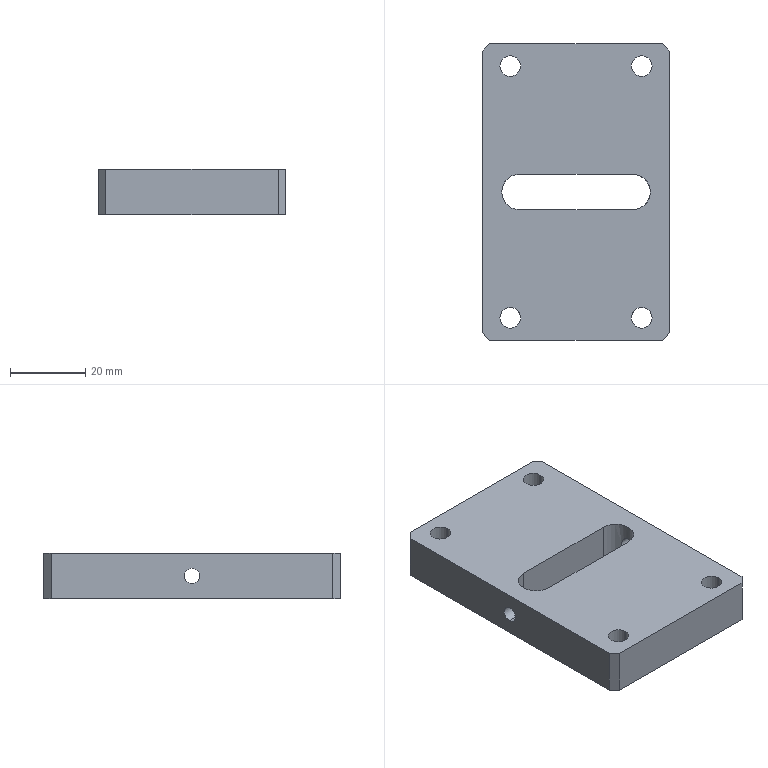Part | SolidWorks | features HoleWzd 3, Chamfer 1, Extrusion 1 | 1 solid | 39 faces | box 50 x 79 x 12 mm | volume 40495 mm3 | cylinder 23 | plane 16 | commonest cylinder face diameters 5.5 x8 10 x8 4.2 x4 9.5 x3
STEP:
#1=CARTESIAN_POINT('',(25.,0.,-2.1));
#2=VERTEX_POINT('',#1);
#3=CARTESIAN_POINT('',(25.,0.,2.1));
#4=VERTEX_POINT('',#3);
#5=CARTESIAN_POINT('',(25.,0.,0.));
#6=DIRECTION('',(-1.,0.,0.));
#7=DIRECTION('',(0.,0.,1.));
#8=AXIS2_PLACEMENT_3D('',#5,#6,#7);
#9=CIRCLE('',#8,2.1);
#10=EDGE_CURVE('',#2,#4,#9,.T.);
#11=ORIENTED_EDGE('',*,*,#10,.F.);
#12=CARTESIAN_POINT('',(19.75,0.,-2.1));
#13=VERTEX_POINT('',#12);
#14=CARTESIAN_POINT('',(-25.,0.,-2.1));
#15=DIRECTION('',(-1.,0.,0.));
#16=VECTOR('',#15,1000.);
#17=LINE('',#14,#16);
#18=EDGE_CURVE('',#2,#13,#17,.T.);
#19=ORIENTED_EDGE('',*,*,#18,.T.);
#20=CARTESIAN_POINT('',(19.75,0.,2.1));
#21=VERTEX_POINT('',#20);
#22=CARTESIAN_POINT('',(19.75,0.,2.1));
#23=CARTESIAN_POINT('',(19.75,-0.1407,2.1));
#24=CARTESIAN_POINT('',(19.744,-0.2787,2.086));
#25=CARTESIAN_POINT('',(19.72,-0.5497,2.031));
#26=CARTESIAN_POINT('',(19.702,-0.6841,1.99));
#27=CARTESIAN_POINT('',(19.658,-0.9378,1.884));
#28=CARTESIAN_POINT('',(19.632,-1.058,1.819));
#29=CARTESIAN_POINT('',(19.574,-1.285,1.667));
#30=CARTESIAN_POINT('',(19.543,-1.391,1.579));
#31=CARTESIAN_POINT('',(19.449,-1.677,1.292));
#32=CARTESIAN_POINT('',(19.384,-1.832,1.062));
#33=CARTESIAN_POINT('',(19.313,-1.99,0.684));
#34=CARTESIAN_POINT('',(19.294,-2.031,0.55));
#35=CARTESIAN_POINT('',(19.267,-2.086,0.2781));
#36=CARTESIAN_POINT('',(19.261,-2.1,0.1406));
#37=CARTESIAN_POINT('',(19.261,-2.1,-0.1376));
#38=CARTESIAN_POINT('',(19.268,-2.086,-0.2786));
#39=CARTESIAN_POINT('',(19.294,-2.031,-0.5497));
#40=CARTESIAN_POINT('',(19.313,-1.991,-0.6823));
#41=CARTESIAN_POINT('',(19.361,-1.884,-0.9374));
#42=CARTESIAN_POINT('',(19.388,-1.819,-1.057));
#43=CARTESIAN_POINT('',(19.448,-1.668,-1.283));
#44=CARTESIAN_POINT('',(19.481,-1.58,-1.39));
#45=CARTESIAN_POINT('',(19.544,-1.389,-1.581));
#46=CARTESIAN_POINT('',(19.575,-1.284,-1.667));
#47=CARTESIAN_POINT('',(19.632,-1.057,-1.82));
#48=CARTESIAN_POINT('',(19.659,-0.9355,-1.885));
#49=CARTESIAN_POINT('',(19.724,-0.5571,-2.043));
#50=CARTESIAN_POINT('',(19.75,-0.2773,-2.1));
#51=CARTESIAN_POINT('',(19.75,0.,-2.1));
#52=B_SPLINE_CURVE_WITH_KNOTS('',3,(#22,#23,#24,#25,#26,#27,#28,#29,#30,#31,#32,#33,#34,#35,#36,#37,#38,#39,#40,#41,#42,#43,#44,#45,#46,#47,#48,#49,#50,#51),.UNSPECIFIED.,.F.,.F.,(4,2,2,2,2,2,2,2,2,2,2,2,2,2,4),(0.,0.0004158,0.0008316,0.001247,0.001663,0.002495,0.002911,0.003326,0.003742,0.004158,0.004574,0.00499,0.005405,0.005821,0.006653),.UNSPECIFIED.);
#53=EDGE_CURVE('',#21,#13,#52,.T.);
#54=ORIENTED_EDGE('',*,*,#53,.F.);
#55=CARTESIAN_POINT('',(-25.,0.,2.1));
#56=DIRECTION('',(-1.,0.,0.));
#57=VECTOR('',#56,1000.);
#58=LINE('',#55,#57);
#59=EDGE_CURVE('',#4,#21,#58,.T.);
#60=ORIENTED_EDGE('',*,*,#59,.F.);
#61=EDGE_LOOP('',(#11,#19,#54,#60));
#62=FACE_OUTER_BOUND('',#61,.T.);
#63=CARTESIAN_POINT('',(-25.,0.,0.));
#64=DIRECTION('',(-1.,0.,0.));
#65=DIRECTION('',(0.,0.,1.));
#66=AXIS2_PLACEMENT_3D('',#63,#64,#65);
#67=CYLINDRICAL_SURFACE('',#66,2.1);
#68=ADVANCED_FACE('',(#62),#67,.F.);
#69=CARTESIAN_POINT('',(-19.75,0.,-2.1));
#70=VERTEX_POINT('',#69);
#71=CARTESIAN_POINT('',(-19.75,0.,2.1));
#72=VERTEX_POINT('',#71);
#73=CARTESIAN_POINT('',(-19.75,0.,-2.1));
#74=CARTESIAN_POINT('',(-19.75,-0.1385,-2.1));
#75=CARTESIAN_POINT('',(-19.744,-0.2793,-2.086));
#76=CARTESIAN_POINT('',(-19.72,-0.5513,-2.031));
#77=CARTESIAN_POINT('',(-19.702,-0.6829,-1.991));
#78=CARTESIAN_POINT('',(-19.636,-1.065,-1.831));
#79=CARTESIAN_POINT('',(-19.575,-1.294,-1.676));
#80=CARTESIAN_POINT('',(-19.48,-1.583,-1.387));
#81=CARTESIAN_POINT('',(-19.448,-1.668,-1.283));
#82=CARTESIAN_POINT('',(-19.389,-1.819,-1.057));
#83=CARTESIAN_POINT('',(-19.36,-1.885,-0.9352));
#84=CARTESIAN_POINT('',(-19.313,-1.991,-0.6828));
#85=CARTESIAN_POINT('',(-19.294,-2.031,-0.552));
#86=CARTESIAN_POINT('',(-19.268,-2.086,-0.2803));
#87=CARTESIAN_POINT('',(-19.261,-2.1,-0.1395));
#88=CARTESIAN_POINT('',(-19.261,-2.1,0.276));
#89=CARTESIAN_POINT('',(-19.289,-2.044,0.5553));
#90=CARTESIAN_POINT('',(-19.36,-1.885,0.935));
#91=CARTESIAN_POINT('',(-19.388,-1.82,1.057));
#92=CARTESIAN_POINT('',(-19.448,-1.668,1.283));
#93=CARTESIAN_POINT('',(-19.48,-1.582,1.387));
#94=CARTESIAN_POINT('',(-19.575,-1.293,1.677));
#95=CARTESIAN_POINT('',(-19.636,-1.066,1.831));
#96=CARTESIAN_POINT('',(-19.702,-0.6831,1.991));
#97=CARTESIAN_POINT('',(-19.72,-0.5517,2.031));
#98=CARTESIAN_POINT('',(-19.744,-0.2812,2.086));
#99=CARTESIAN_POINT('',(-19.75,-0.1406,2.1));
#100=CARTESIAN_POINT('',(-19.75,0.,2.1));
#101=B_SPLINE_CURVE_WITH_KNOTS('',3,(#73,#74,#75,#76,#77,#78,#79,#80,#81,#82,#83,#84,#85,#86,#87,#88,#89,#90,#91,#92,#93,#94,#95,#96,#97,#98,#99,#100),.UNSPECIFIED.,.F.,.F.,(4,2,2,2,2,2,2,2,2,2,2,2,2,4),(0.006653,0.007068,0.007483,0.008314,0.00873,0.009145,0.00956,0.009976,0.01081,0.01122,0.01164,0.01247,0.01288,0.0133),.UNSPECIFIED.);
#102=EDGE_CURVE('',#70,#72,#101,.T.);
#103=ORIENTED_EDGE('',*,*,#102,.F.);
#104=CARTESIAN_POINT('',(-25.,0.,-2.1));
#105=VERTEX_POINT('',#104);
#106=CARTESIAN_POINT('',(-25.,0.,-2.1));
#107=DIRECTION('',(-1.,0.,0.));
#108=VECTOR('',#107,1000.);
#109=LINE('',#106,#108);
#110=EDGE_CURVE('',#70,#105,#109,.T.);
#111=ORIENTED_EDGE('',*,*,#110,.T.);
#112=CARTESIAN_POINT('',(-25.,0.,2.1));
#113=VERTEX_POINT('',#112);
#114=CARTESIAN_POINT('',(-25.,0.,0.));
#115=DIRECTION('',(-1.,0.,0.));
#116=DIRECTION('',(0.,0.,1.));
#117=AXIS2_PLACEMENT_3D('',#114,#115,#116);
#118=CIRCLE('',#117,2.1);
#119=EDGE_CURVE('',#105,#113,#118,.T.);
#120=ORIENTED_EDGE('',*,*,#119,.T.);
#121=CARTESIAN_POINT('',(-25.,0.,2.1));
#122=DIRECTION('',(-1.,0.,0.));
#123=VECTOR('',#122,1000.);
#124=LINE('',#121,#123);
#125=EDGE_CURVE('',#72,#113,#124,.T.);
#126=ORIENTED_EDGE('',*,*,#125,.F.);
#127=EDGE_LOOP('',(#103,#111,#120,#126));
#128=FACE_OUTER_BOUND('',#127,.T.);
#129=CARTESIAN_POINT('',(-25.,0.,0.));
#130=DIRECTION('',(-1.,0.,0.));
#131=DIRECTION('',(0.,0.,1.));
#132=AXIS2_PLACEMENT_3D('',#129,#130,#131);
#133=CYLINDRICAL_SURFACE('',#132,2.1);
#134=ADVANCED_FACE('',(#128),#133,.F.);
#135=CARTESIAN_POINT('',(-12.5,33.5,-0.3));
#136=VERTEX_POINT('',#135);
#137=CARTESIAN_POINT('',(-22.5,33.5,-0.3));
#138=VERTEX_POINT('',#137);
#139=CARTESIAN_POINT('',(-17.5,33.5,-0.3));
#140=DIRECTION('',(0.,0.,-1.));
#141=DIRECTION('',(-1.,0.,0.));
#142=AXIS2_PLACEMENT_3D('',#139,#140,#141);
#143=CIRCLE('',#142,5.);
#144=EDGE_CURVE('',#136,#138,#143,.T.);
#145=ORIENTED_EDGE('',*,*,#144,.F.);
#146=CARTESIAN_POINT('',(-12.5,33.5,-6.));
#147=VERTEX_POINT('',#146);
#148=CARTESIAN_POINT('',(-12.5,33.5,-6.));
#149=DIRECTION('',(0.,0.,-1.));
#150=VECTOR('',#149,1000.);
#151=LINE('',#148,#150);
#152=EDGE_CURVE('',#136,#147,#151,.T.);
#153=ORIENTED_EDGE('',*,*,#152,.T.);
#154=CARTESIAN_POINT('',(-22.5,33.5,-6.));
#155=VERTEX_POINT('',#154);
#156=CARTESIAN_POINT('',(-17.5,33.5,-6.));
#157=DIRECTION('',(0.,0.,-1.));
#158=DIRECTION('',(-1.,0.,0.));
#159=AXIS2_PLACEMENT_3D('',#156,#157,#158);
#160=CIRCLE('',#159,5.);
#161=EDGE_CURVE('',#147,#155,#160,.T.);
#162=ORIENTED_EDGE('',*,*,#161,.T.);
#163=CARTESIAN_POINT('',(-22.5,33.5,-6.));
#164=DIRECTION('',(0.,0.,-1.));
#165=VECTOR('',#164,1000.);
#166=LINE('',#163,#165);
#167=EDGE_CURVE('',#138,#155,#166,.T.);
#168=ORIENTED_EDGE('',*,*,#167,.F.);
#169=EDGE_LOOP('',(#145,#153,#162,#168));
#170=FACE_OUTER_BOUND('',#169,.T.);
#171=CARTESIAN_POINT('',(-17.5,33.5,-6.));
#172=DIRECTION('',(0.,0.,-1.));
#173=DIRECTION('',(-1.,0.,0.));
#174=AXIS2_PLACEMENT_3D('',#171,#172,#173);
#175=CYLINDRICAL_SURFACE('',#174,5.);
#176=ADVANCED_FACE('',(#170),#175,.F.);
#177=CARTESIAN_POINT('',(-14.75,33.5,6.));
#178=VERTEX_POINT('',#177);
#179=CARTESIAN_POINT('',(-20.25,33.5,6.));
#180=VERTEX_POINT('',#179);
#181=CARTESIAN_POINT('',(-17.5,33.5,6.));
#182=DIRECTION('',(0.,0.,-1.));
#183=DIRECTION('',(-1.,0.,0.));
#184=AXIS2_PLACEMENT_3D('',#181,#182,#183);
#185=CIRCLE('',#184,2.75);
#186=EDGE_CURVE('',#178,#180,#185,.T.);
#187=ORIENTED_EDGE('',*,*,#186,.F.);
#188=CARTESIAN_POINT('',(-14.75,33.5,-0.3));
#189=VERTEX_POINT('',#188);
#190=CARTESIAN_POINT('',(-14.75,33.5,-6.));
#191=DIRECTION('',(0.,0.,-1.));
#192=VECTOR('',#191,1000.);
#193=LINE('',#190,#192);
#194=EDGE_CURVE('',#178,#189,#193,.T.);
#195=ORIENTED_EDGE('',*,*,#194,.T.);
#196=CARTESIAN_POINT('',(-20.25,33.5,-0.3));
#197=VERTEX_POINT('',#196);
#198=CARTESIAN_POINT('',(-17.5,33.5,-0.3));
#199=DIRECTION('',(0.,0.,-1.));
#200=DIRECTION('',(-1.,0.,0.));
#201=AXIS2_PLACEMENT_3D('',#198,#199,#200);
#202=CIRCLE('',#201,2.75);
#203=EDGE_CURVE('',#189,#197,#202,.T.);
#204=ORIENTED_EDGE('',*,*,#203,.T.);
#205=CARTESIAN_POINT('',(-20.25,33.5,-6.));
#206=DIRECTION('',(0.,0.,-1.));
#207=VECTOR('',#206,1000.);
#208=LINE('',#205,#207);
#209=EDGE_CURVE('',#180,#197,#208,.T.);
#210=ORIENTED_EDGE('',*,*,#209,.F.);
#211=EDGE_LOOP('',(#187,#195,#204,#210));
#212=FACE_OUTER_BOUND('',#211,.T.);
#213=CARTESIAN_POINT('',(-17.5,33.5,-6.));
#214=DIRECTION('',(0.,0.,-1.));
#215=DIRECTION('',(-1.,0.,0.));
#216=AXIS2_PLACEMENT_3D('',#213,#214,#215);
#217=CYLINDRICAL_SURFACE('',#216,2.75);
#218=ADVANCED_FACE('',(#212),#217,.F.);
#219=CARTESIAN_POINT('',(22.5,33.5,-0.3));
#220=VERTEX_POINT('',#219);
#221=CARTESIAN_POINT('',(12.5,33.5,-0.3));
#222=VERTEX_POINT('',#221);
#223=CARTESIAN_POINT('',(17.5,33.5,-0.3));
#224=DIRECTION('',(0.,0.,-1.));
#225=DIRECTION('',(-1.,0.,0.));
#226=AXIS2_PLACEMENT_3D('',#223,#224,#225);
#227=CIRCLE('',#226,5.);
#228=EDGE_CURVE('',#220,#222,#227,.T.);
#229=ORIENTED_EDGE('',*,*,#228,.F.);
#230=CARTESIAN_POINT('',(22.5,33.5,-6.));
#231=VERTEX_POINT('',#230);
#232=CARTESIAN_POINT('',(22.5,33.5,-6.));
#233=DIRECTION('',(0.,0.,-1.));
#234=VECTOR('',#233,1000.);
#235=LINE('',#232,#234);
#236=EDGE_CURVE('',#220,#231,#235,.T.);
#237=ORIENTED_EDGE('',*,*,#236,.T.);
#238=CARTESIAN_POINT('',(12.5,33.5,-6.));
#239=VERTEX_POINT('',#238);
#240=CARTESIAN_POINT('',(17.5,33.5,-6.));
#241=DIRECTION('',(0.,0.,-1.));
#242=DIRECTION('',(-1.,0.,0.));
#243=AXIS2_PLACEMENT_3D('',#240,#241,#242);
#244=CIRCLE('',#243,5.);
#245=EDGE_CURVE('',#231,#239,#244,.T.);
#246=ORIENTED_EDGE('',*,*,#245,.T.);
#247=CARTESIAN_POINT('',(12.5,33.5,-6.));
#248=DIRECTION('',(0.,0.,-1.));
#249=VECTOR('',#248,1000.);
#250=LINE('',#247,#249);
#251=EDGE_CURVE('',#222,#239,#250,.T.);
#252=ORIENTED_EDGE('',*,*,#251,.F.);
#253=EDGE_LOOP('',(#229,#237,#246,#252));
#254=FACE_OUTER_BOUND('',#253,.T.);
#255=CARTESIAN_POINT('',(17.5,33.5,-6.));
#256=DIRECTION('',(0.,0.,-1.));
#257=DIRECTION('',(-1.,0.,0.));
#258=AXIS2_PLACEMENT_3D('',#255,#256,#257);
#259=CYLINDRICAL_SURFACE('',#258,5.);
#260=ADVANCED_FACE('',(#254),#259,.F.);
#261=CARTESIAN_POINT('',(20.25,33.5,6.));
#262=VERTEX_POINT('',#261);
#263=CARTESIAN_POINT('',(14.75,33.5,6.));
#264=VERTEX_POINT('',#263);
#265=CARTESIAN_POINT('',(17.5,33.5,6.));
#266=DIRECTION('',(0.,0.,-1.));
#267=DIRECTION('',(-1.,0.,0.));
#268=AXIS2_PLACEMENT_3D('',#265,#266,#267);
#269=CIRCLE('',#268,2.75);
#270=EDGE_CURVE('',#262,#264,#269,.T.);
#271=ORIENTED_EDGE('',*,*,#270,.F.);
#272=CARTESIAN_POINT('',(20.25,33.5,-0.3));
#273=VERTEX_POINT('',#272);
#274=CARTESIAN_POINT('',(20.25,33.5,-6.));
#275=DIRECTION('',(0.,0.,-1.));
#276=VECTOR('',#275,1000.);
#277=LINE('',#274,#276);
#278=EDGE_CURVE('',#262,#273,#277,.T.);
#279=ORIENTED_EDGE('',*,*,#278,.T.);
#280=CARTESIAN_POINT('',(14.75,33.5,-0.3));
#281=VERTEX_POINT('',#280);
#282=CARTESIAN_POINT('',(17.5,33.5,-0.3));
#283=DIRECTION('',(0.,0.,-1.));
#284=DIRECTION('',(-1.,0.,0.));
#285=AXIS2_PLACEMENT_3D('',#282,#283,#284);
#286=CIRCLE('',#285,2.75);
#287=EDGE_CURVE('',#273,#281,#286,.T.);
#288=ORIENTED_EDGE('',*,*,#287,.T.);
#289=CARTESIAN_POINT('',(14.75,33.5,-6.));
#290=DIRECTION('',(0.,0.,-1.));
#291=VECTOR('',#290,1000.);
#292=LINE('',#289,#291);
#293=EDGE_CURVE('',#264,#281,#292,.T.);
#294=ORIENTED_EDGE('',*,*,#293,.F.);
#295=EDGE_LOOP('',(#271,#279,#288,#294));
#296=FACE_OUTER_BOUND('',#295,.T.);
#297=CARTESIAN_POINT('',(17.5,33.5,-6.));
#298=DIRECTION('',(0.,0.,-1.));
#299=DIRECTION('',(-1.,0.,0.));
#300=AXIS2_PLACEMENT_3D('',#297,#298,#299);
#301=CYLINDRICAL_SURFACE('',#300,2.75);
#302=ADVANCED_FACE('',(#296),#301,.F.);
#303=CARTESIAN_POINT('',(-12.5,-33.5,-0.3));
#304=VERTEX_POINT('',#303);
#305=CARTESIAN_POINT('',(-22.5,-33.5,-0.3));
#306=VERTEX_POINT('',#305);
#307=CARTESIAN_POINT('',(-17.5,-33.5,-0.3));
#308=DIRECTION('',(0.,0.,-1.));
#309=DIRECTION('',(-1.,0.,0.));
#310=AXIS2_PLACEMENT_3D('',#307,#308,#309);
#311=CIRCLE('',#310,5.);
#312=EDGE_CURVE('',#304,#306,#311,.T.);
#313=ORIENTED_EDGE('',*,*,#312,.F.);
#314=CARTESIAN_POINT('',(-12.5,-33.5,-6.));
#315=VERTEX_POINT('',#314);
#316=CARTESIAN_POINT('',(-12.5,-33.5,-6.));
#317=DIRECTION('',(0.,0.,-1.));
#318=VECTOR('',#317,1000.);
#319=LINE('',#316,#318);
#320=EDGE_CURVE('',#304,#315,#319,.T.);
#321=ORIENTED_EDGE('',*,*,#320,.T.);
#322=CARTESIAN_POINT('',(-22.5,-33.5,-6.));
#323=VERTEX_POINT('',#322);
#324=CARTESIAN_POINT('',(-17.5,-33.5,-6.));
#325=DIRECTION('',(0.,0.,-1.));
#326=DIRECTION('',(-1.,0.,0.));
#327=AXIS2_PLACEMENT_3D('',#324,#325,#326);
#328=CIRCLE('',#327,5.);
#329=EDGE_CURVE('',#315,#323,#328,.T.);
#330=ORIENTED_EDGE('',*,*,#329,.T.);
#331=CARTESIAN_POINT('',(-22.5,-33.5,-6.));
#332=DIRECTION('',(0.,0.,-1.));
#333=VECTOR('',#332,1000.);
#334=LINE('',#331,#333);
#335=EDGE_CURVE('',#306,#323,#334,.T.);
#336=ORIENTED_EDGE('',*,*,#335,.F.);
#337=EDGE_LOOP('',(#313,#321,#330,#336));
#338=FACE_OUTER_BOUND('',#337,.T.);
#339=CARTESIAN_POINT('',(-17.5,-33.5,-6.));
#340=DIRECTION('',(0.,0.,-1.));
#341=DIRECTION('',(-1.,0.,0.));
#342=AXIS2_PLACEMENT_3D('',#339,#340,#341);
#343=CYLINDRICAL_SURFACE('',#342,5.);
#344=ADVANCED_FACE('',(#338),#343,.F.);
#345=CARTESIAN_POINT('',(-14.75,-33.5,6.));
#346=VERTEX_POINT('',#345);
#347=CARTESIAN_POINT('',(-20.25,-33.5,6.));
#348=VERTEX_POINT('',#347);
#349=CARTESIAN_POINT('',(-17.5,-33.5,6.));
#350=DIRECTION('',(0.,0.,-1.));
#351=DIRECTION('',(-1.,0.,0.));
#352=AXIS2_PLACEMENT_3D('',#349,#350,#351);
#353=CIRCLE('',#352,2.75);
#354=EDGE_CURVE('',#346,#348,#353,.T.);
#355=ORIENTED_EDGE('',*,*,#354,.F.);
#356=CARTESIAN_POINT('',(-14.75,-33.5,-0.3));
#357=VERTEX_POINT('',#356);
#358=CARTESIAN_POINT('',(-14.75,-33.5,-6.));
#359=DIRECTION('',(0.,0.,-1.));
#360=VECTOR('',#359,1000.);
#361=LINE('',#358,#360);
#362=EDGE_CURVE('',#346,#357,#361,.T.);
#363=ORIENTED_EDGE('',*,*,#362,.T.);
#364=CARTESIAN_POINT('',(-20.25,-33.5,-0.3));
#365=VERTEX_POINT('',#364);
#366=CARTESIAN_POINT('',(-17.5,-33.5,-0.3));
#367=DIRECTION('',(0.,0.,-1.));
#368=DIRECTION('',(-1.,0.,0.));
#369=AXIS2_PLACEMENT_3D('',#366,#367,#368);
#370=CIRCLE('',#369,2.75);
#371=EDGE_CURVE('',#357,#365,#370,.T.);
#372=ORIENTED_EDGE('',*,*,#371,.T.);
#373=CARTESIAN_POINT('',(-20.25,-33.5,-6.));
#374=DIRECTION('',(0.,0.,-1.));
#375=VECTOR('',#374,1000.);
#376=LINE('',#373,#375);
#377=EDGE_CURVE('',#348,#365,#376,.T.);
#378=ORIENTED_EDGE('',*,*,#377,.F.);
#379=EDGE_LOOP('',(#355,#363,#372,#378));
#380=FACE_OUTER_BOUND('',#379,.T.);
#381=CARTESIAN_POINT('',(-17.5,-33.5,-6.));
#382=DIRECTION('',(0.,0.,-1.));
#383=DIRECTION('',(-1.,0.,0.));
#384=AXIS2_PLACEMENT_3D('',#381,#382,#383);
#385=CYLINDRICAL_SURFACE('',#384,2.75);
#386=ADVANCED_FACE('',(#380),#385,.F.);
#387=CARTESIAN_POINT('',(22.5,-33.5,-0.3));
#388=VERTEX_POINT('',#387);
#389=CARTESIAN_POINT('',(12.5,-33.5,-0.3));
#390=VERTEX_POINT('',#389);
#391=CARTESIAN_POINT('',(17.5,-33.5,-0.3));
#392=DIRECTION('',(0.,0.,-1.));
#393=DIRECTION('',(-1.,0.,0.));
#394=AXIS2_PLACEMENT_3D('',#391,#392,#393);
#395=CIRCLE('',#394,5.);
#396=EDGE_CURVE('',#388,#390,#395,.T.);
#397=ORIENTED_EDGE('',*,*,#396,.F.);
#398=CARTESIAN_POINT('',(22.5,-33.5,-6.));
#399=VERTEX_POINT('',#398);
#400=CARTESIAN_POINT('',(22.5,-33.5,-6.));
#401=DIRECTION('',(0.,0.,-1.));
#402=VECTOR('',#401,1000.);
#403=LINE('',#400,#402);
#404=EDGE_CURVE('',#388,#399,#403,.T.);
#405=ORIENTED_EDGE('',*,*,#404,.T.);
#406=CARTESIAN_POINT('',(12.5,-33.5,-6.));
#407=VERTEX_POINT('',#406);
#408=CARTESIAN_POINT('',(17.5,-33.5,-6.));
#409=DIRECTION('',(0.,0.,-1.));
#410=DIRECTION('',(-1.,0.,0.));
#411=AXIS2_PLACEMENT_3D('',#408,#409,#410);
#412=CIRCLE('',#411,5.);
#413=EDGE_CURVE('',#399,#407,#412,.T.);
#414=ORIENTED_EDGE('',*,*,#413,.T.);
#415=CARTESIAN_POINT('',(12.5,-33.5,-6.));
#416=DIRECTION('',(0.,0.,-1.));
#417=VECTOR('',#416,1000.);
#418=LINE('',#415,#417);
#419=EDGE_CURVE('',#390,#407,#418,.T.);
#420=ORIENTED_EDGE('',*,*,#419,.F.);
#421=EDGE_LOOP('',(#397,#405,#414,#420));
#422=FACE_OUTER_BOUND('',#421,.T.);
#423=CARTESIAN_POINT('',(17.5,-33.5,-6.));
#424=DIRECTION('',(0.,0.,-1.));
#425=DIRECTION('',(-1.,0.,0.));
#426=AXIS2_PLACEMENT_3D('',#423,#424,#425);
#427=CYLINDRICAL_SURFACE('',#426,5.);
#428=ADVANCED_FACE('',(#422),#427,.F.);
#429=CARTESIAN_POINT('',(20.25,-33.5,6.));
#430=VERTEX_POINT('',#429);
#431=CARTESIAN_POINT('',(14.75,-33.5,6.));
#432=VERTEX_POINT('',#431);
#433=CARTESIAN_POINT('',(17.5,-33.5,6.));
#434=DIRECTION('',(0.,0.,-1.));
#435=DIRECTION('',(-1.,0.,0.));
#436=AXIS2_PLACEMENT_3D('',#433,#434,#435);
#437=CIRCLE('',#436,2.75);
#438=EDGE_CURVE('',#430,#432,#437,.T.);
#439=ORIENTED_EDGE('',*,*,#438,.F.);
#440=CARTESIAN_POINT('',(20.25,-33.5,-0.3));
#441=VERTEX_POINT('',#440);
#442=CARTESIAN_POINT('',(20.25,-33.5,-6.));
#443=DIRECTION('',(0.,0.,-1.));
#444=VECTOR('',#443,1000.);
#445=LINE('',#442,#444);
#446=EDGE_CURVE('',#430,#441,#445,.T.);
#447=ORIENTED_EDGE('',*,*,#446,.T.);
#448=CARTESIAN_POINT('',(14.75,-33.5,-0.3));
#449=VERTEX_POINT('',#448);
#450=CARTESIAN_POINT('',(17.5,-33.5,-0.3));
#451=DIRECTION('',(0.,0.,-1.));
#452=DIRECTION('',(-1.,0.,0.));
#453=AXIS2_PLACEMENT_3D('',#450,#451,#452);
#454=CIRCLE('',#453,2.75);
#455=EDGE_CURVE('',#441,#449,#454,.T.);
#456=ORIENTED_EDGE('',*,*,#455,.T.);
#457=CARTESIAN_POINT('',(14.75,-33.5,-6.));
#458=DIRECTION('',(0.,0.,-1.));
#459=VECTOR('',#458,1000.);
#460=LINE('',#457,#459);
#461=EDGE_CURVE('',#432,#449,#460,.T.);
#462=ORIENTED_EDGE('',*,*,#461,.F.);
#463=EDGE_LOOP('',(#439,#447,#456,#462));
#464=FACE_OUTER_BOUND('',#463,.T.);
#465=CARTESIAN_POINT('',(17.5,-33.5,-6.));
#466=DIRECTION('',(0.,0.,-1.));
#467=DIRECTION('',(-1.,0.,0.));
#468=AXIS2_PLACEMENT_3D('',#465,#466,#467);
#469=CYLINDRICAL_SURFACE('',#468,2.75);
#470=ADVANCED_FACE('',(#464),#469,.F.);
#471=CARTESIAN_POINT('',(-19.75,0.,6.));
#472=VERTEX_POINT('',#471);
#473=CARTESIAN_POINT('',(-15.,4.75,6.));
#474=VERTEX_POINT('',#473);
#475=CARTESIAN_POINT('',(-15.,0.,6.));
#476=DIRECTION('',(0.,0.,-1.));
#477=DIRECTION('',(-1.,0.,0.));
#478=AXIS2_PLACEMENT_3D('',#475,#476,#477);
#479=CIRCLE('',#478,4.75);
#480=EDGE_CURVE('',#472,#474,#479,.T.);
#481=ORIENTED_EDGE('',*,*,#480,.F.);
#482=CARTESIAN_POINT('',(-19.75,0.,-6.));
#483=DIRECTION('',(0.,0.,-1.));
#484=VECTOR('',#483,1000.);
#485=LINE('',#482,#484);
#486=EDGE_CURVE('',#472,#72,#485,.T.);
#487=ORIENTED_EDGE('',*,*,#486,.T.);
#488=CARTESIAN_POINT('',(-19.75,0.,2.1));
#489=CARTESIAN_POINT('',(-19.75,0.1407,2.1));
#490=CARTESIAN_POINT('',(-19.744,0.2787,2.086));
#491=CARTESIAN_POINT('',(-19.72,0.5497,2.031));
#492=CARTESIAN_POINT('',(-19.702,0.6841,1.99));
#493=CARTESIAN_POINT('',(-19.658,0.9378,1.884));
#494=CARTESIAN_POINT('',(-19.632,1.058,1.819));
#495=CARTESIAN_POINT('',(-19.574,1.285,1.667));
#496=CARTESIAN_POINT('',(-19.543,1.391,1.579));
#497=CARTESIAN_POINT('',(-19.449,1.677,1.292));
#498=CARTESIAN_POINT('',(-19.384,1.832,1.062));
#499=CARTESIAN_POINT('',(-19.313,1.99,0.684));
#500=CARTESIAN_POINT('',(-19.294,2.031,0.55));
#501=CARTESIAN_POINT('',(-19.267,2.086,0.2781));
#502=CARTESIAN_POINT('',(-19.261,2.1,0.1406));
#503=CARTESIAN_POINT('',(-19.261,2.1,-0.1376));
#504=CARTESIAN_POINT('',(-19.268,2.086,-0.2786));
#505=CARTESIAN_POINT('',(-19.294,2.031,-0.5497));
#506=CARTESIAN_POINT('',(-19.313,1.991,-0.6823));
#507=CARTESIAN_POINT('',(-19.361,1.884,-0.9374));
#508=CARTESIAN_POINT('',(-19.388,1.819,-1.057));
#509=CARTESIAN_POINT('',(-19.448,1.668,-1.283));
#510=CARTESIAN_POINT('',(-19.481,1.58,-1.39));
#511=CARTESIAN_POINT('',(-19.544,1.389,-1.581));
#512=CARTESIAN_POINT('',(-19.575,1.284,-1.667));
#513=CARTESIAN_POINT('',(-19.632,1.057,-1.82));
#514=CARTESIAN_POINT('',(-19.659,0.9355,-1.885));
#515=CARTESIAN_POINT('',(-19.724,0.5571,-2.043));
#516=CARTESIAN_POINT('',(-19.75,0.2773,-2.1));
#517=CARTESIAN_POINT('',(-19.75,0.,-2.1));
#518=B_SPLINE_CURVE_WITH_KNOTS('',3,(#488,#489,#490,#491,#492,#493,#494,#495,#496,#497,#498,#499,#500,#501,#502,#503,#504,#505,#506,#507,#508,#509,#510,#511,#512,#513,#514,#515,#516,#517),.UNSPECIFIED.,.F.,.F.,(4,2,2,2,2,2,2,2,2,2,2,2,2,2,4),(0.,0.0004158,0.0008316,0.001247,0.001663,0.002495,0.002911,0.003326,0.003742,0.004158,0.004574,0.00499,0.005405,0.005821,0.006653),.UNSPECIFIED.);
#519=EDGE_CURVE('',#72,#70,#518,.T.);
#520=ORIENTED_EDGE('',*,*,#519,.T.);
#521=CARTESIAN_POINT('',(-19.75,0.,-6.));
#522=VERTEX_POINT('',#521);
#523=CARTESIAN_POINT('',(-19.75,0.,-6.));
#524=DIRECTION('',(0.,0.,-1.));
#525=VECTOR('',#524,1000.);
#526=LINE('',#523,#525);
#527=EDGE_CURVE('',#70,#522,#526,.T.);
#528=ORIENTED_EDGE('',*,*,#527,.T.);
#529=CARTESIAN_POINT('',(-15.,4.75,-6.));
#530=VERTEX_POINT('',#529);
#531=CARTESIAN_POINT('',(-15.,0.,-6.));
#532=DIRECTION('',(0.,0.,-1.));
#533=DIRECTION('',(-1.,0.,0.));
#534=AXIS2_PLACEMENT_3D('',#531,#532,#533);
#535=CIRCLE('',#534,4.75);
#536=EDGE_CURVE('',#522,#530,#535,.T.);
#537=ORIENTED_EDGE('',*,*,#536,.T.);
#538=CARTESIAN_POINT('',(-15.,4.75,-6.));
#539=DIRECTION('',(0.,0.,-1.));
#540=VECTOR('',#539,1000.);
#541=LINE('',#538,#540);
#542=EDGE_CURVE('',#474,#530,#541,.T.);
#543=ORIENTED_EDGE('',*,*,#542,.F.);
#544=EDGE_LOOP('',(#481,#487,#520,#528,#537,#543));
#545=FACE_OUTER_BOUND('',#544,.T.);
#546=CARTESIAN_POINT('',(-15.,0.,-6.));
#547=DIRECTION('',(0.,0.,-1.));
#548=DIRECTION('',(-1.,0.,0.));
#549=AXIS2_PLACEMENT_3D('',#546,#547,#548);
#550=CYLINDRICAL_SURFACE('',#549,4.75);
#551=ADVANCED_FACE('',(#545),#550,.F.);
#552=CARTESIAN_POINT('',(25.,0.,0.));
#553=DIRECTION('',(-1.,0.,0.));
#554=DIRECTION('',(0.,0.,1.));
#555=AXIS2_PLACEMENT_3D('',#552,#553,#554);
#556=CIRCLE('',#555,2.1);
#557=EDGE_CURVE('',#4,#2,#556,.T.);
#558=ORIENTED_EDGE('',*,*,#557,.T.);
#559=ORIENTED_EDGE('',*,*,#10,.T.);
#560=EDGE_LOOP('',(#558,#559));
#561=FACE_BOUND('',#560,.T.);
#562=CARTESIAN_POINT('',(25.,-37.5,6.));
#563=VERTEX_POINT('',#562);
#564=CARTESIAN_POINT('',(25.,37.5,6.));
#565=VERTEX_POINT('',#564);
#566=CARTESIAN_POINT('',(25.,-39.5,6.));
#567=DIRECTION('',(0.,1.,0.));
#568=VECTOR('',#567,1000.);
#569=LINE('',#566,#568);
#570=EDGE_CURVE('',#563,#565,#569,.T.);
#571=ORIENTED_EDGE('',*,*,#570,.F.);
#572=CARTESIAN_POINT('',(25.,-37.5,-6.));
#573=VERTEX_POINT('',#572);
#574=CARTESIAN_POINT('',(25.,-37.5,6.));
#575=DIRECTION('',(0.,0.,-1.));
#576=VECTOR('',#575,1000.);
#577=LINE('',#574,#576);
#578=EDGE_CURVE('',#563,#573,#577,.T.);
#579=ORIENTED_EDGE('',*,*,#578,.T.);
#580=CARTESIAN_POINT('',(25.,37.5,-6.));
#581=VERTEX_POINT('',#580);
#582=CARTESIAN_POINT('',(25.,-39.5,-6.));
#583=DIRECTION('',(0.,1.,0.));
#584=VECTOR('',#583,1000.);
#585=LINE('',#582,#584);
#586=EDGE_CURVE('',#573,#581,#585,.T.);
#587=ORIENTED_EDGE('',*,*,#586,.T.);
#588=CARTESIAN_POINT('',(25.,37.5,6.));
#589=DIRECTION('',(0.,0.,1.));
#590=VECTOR('',#589,1000.);
#591=LINE('',#588,#590);
#592=EDGE_CURVE('',#581,#565,#591,.T.);
#593=ORIENTED_EDGE('',*,*,#592,.T.);
#594=EDGE_LOOP('',(#571,#579,#587,#593));
#595=FACE_OUTER_BOUND('',#594,.T.);
#596=CARTESIAN_POINT('',(25.,-39.5,6.));
#597=DIRECTION('',(-1.,0.,0.));
#598=DIRECTION('',(0.,0.,1.));
#599=AXIS2_PLACEMENT_3D('',#596,#597,#598);
#600=PLANE('',#599);
#601=ADVANCED_FACE('',(#561,#595),#600,.F.);
#602=CARTESIAN_POINT('',(23.,39.5,-6.));
#603=VERTEX_POINT('',#602);
#604=CARTESIAN_POINT('',(-23.,39.5,-6.));
#605=VERTEX_POINT('',#604);
#606=CARTESIAN_POINT('',(-25.,39.5,-6.));
#607=DIRECTION('',(-1.,0.,0.));
#608=VECTOR('',#607,1000.);
#609=LINE('',#606,#608);
#610=EDGE_CURVE('',#603,#605,#609,.T.);
#611=ORIENTED_EDGE('',*,*,#610,.T.);
#612=CARTESIAN_POINT('',(-23.,39.5,6.));
#613=VERTEX_POINT('',#612);
#614=CARTESIAN_POINT('',(-23.,39.5,6.));
#615=DIRECTION('',(0.,0.,1.));
#616=VECTOR('',#615,1000.);
#617=LINE('',#614,#616);
#618=EDGE_CURVE('',#605,#613,#617,.T.);
#619=ORIENTED_EDGE('',*,*,#618,.T.);
#620=CARTESIAN_POINT('',(23.,39.5,6.));
#621=VERTEX_POINT('',#620);
#622=CARTESIAN_POINT('',(-25.,39.5,6.));
#623=DIRECTION('',(-1.,0.,0.));
#624=VECTOR('',#623,1000.);
#625=LINE('',#622,#624);
#626=EDGE_CURVE('',#621,#613,#625,.T.);
#627=ORIENTED_EDGE('',*,*,#626,.F.);
#628=CARTESIAN_POINT('',(23.,39.5,6.));
#629=DIRECTION('',(0.,0.,-1.));
#630=VECTOR('',#629,1000.);
#631=LINE('',#628,#630);
#632=EDGE_CURVE('',#621,#603,#631,.T.);
#633=ORIENTED_EDGE('',*,*,#632,.T.);
#634=EDGE_LOOP('',(#611,#619,#627,#633));
#635=FACE_OUTER_BOUND('',#634,.T.);
#636=CARTESIAN_POINT('',(-25.,39.5,6.));
#637=DIRECTION('',(0.,-1.,0.));
#638=DIRECTION('',(0.,0.,-1.));
#639=AXIS2_PLACEMENT_3D('',#636,#637,#638);
#640=PLANE('',#639);
#641=ADVANCED_FACE('',(#635),#640,.F.);
#642=CARTESIAN_POINT('',(-25.,0.,0.));
#643=DIRECTION('',(-1.,0.,0.));
#644=DIRECTION('',(0.,0.,1.));
#645=AXIS2_PLACEMENT_3D('',#642,#643,#644);
#646=CIRCLE('',#645,2.1);
#647=EDGE_CURVE('',#113,#105,#646,.T.);
#648=ORIENTED_EDGE('',*,*,#647,.F.);
#649=ORIENTED_EDGE('',*,*,#119,.F.);
#650=EDGE_LOOP('',(#648,#649));
#651=FACE_BOUND('',#650,.T.);
#652=CARTESIAN_POINT('',(-25.,37.5,-6.));
#653=VERTEX_POINT('',#652);
#654=CARTESIAN_POINT('',(-25.,-37.5,-6.));
#655=VERTEX_POINT('',#654);
#656=CARTESIAN_POINT('',(-25.,-39.5,-6.));
#657=DIRECTION('',(0.,-1.,0.));
#658=VECTOR('',#657,1000.);
#659=LINE('',#656,#658);
#660=EDGE_CURVE('',#653,#655,#659,.T.);
#661=ORIENTED_EDGE('',*,*,#660,.T.);
#662=CARTESIAN_POINT('',(-25.,-37.5,6.));
#663=VERTEX_POINT('',#662);
#664=CARTESIAN_POINT('',(-25.,-37.5,6.));
#665=DIRECTION('',(0.,0.,1.));
#666=VECTOR('',#665,1000.);
#667=LINE('',#664,#666);
#668=EDGE_CURVE('',#655,#663,#667,.T.);
#669=ORIENTED_EDGE('',*,*,#668,.T.);
#670=CARTESIAN_POINT('',(-25.,37.5,6.));
#671=VERTEX_POINT('',#670);
#672=CARTESIAN_POINT('',(-25.,-39.5,6.));
#673=DIRECTION('',(0.,-1.,0.));
#674=VECTOR('',#673,1000.);
#675=LINE('',#672,#674);
#676=EDGE_CURVE('',#671,#663,#675,.T.);
#677=ORIENTED_EDGE('',*,*,#676,.F.);
#678=CARTESIAN_POINT('',(-25.,37.5,6.));
#679=DIRECTION('',(0.,0.,-1.));
#680=VECTOR('',#679,1000.);
#681=LINE('',#678,#680);
#682=EDGE_CURVE('',#671,#653,#681,.T.);
#683=ORIENTED_EDGE('',*,*,#682,.T.);
#684=EDGE_LOOP('',(#661,#669,#677,#683));
#685=FACE_OUTER_BOUND('',#684,.T.);
#686=CARTESIAN_POINT('',(-25.,-39.5,6.));
#687=DIRECTION('',(1.,0.,0.));
#688=DIRECTION('',(0.,0.,-1.));
#689=AXIS2_PLACEMENT_3D('',#686,#687,#688);
#690=PLANE('',#689);
#691=ADVANCED_FACE('',(#651,#685),#690,.F.);
#692=CARTESIAN_POINT('',(-23.,-39.5,-6.));
#693=VERTEX_POINT('',#692);
#694=CARTESIAN_POINT('',(23.,-39.5,-6.));
#695=VERTEX_POINT('',#694);
#696=CARTESIAN_POINT('',(-25.,-39.5,-6.));
#697=DIRECTION('',(1.,0.,0.));
#698=VECTOR('',#697,1000.);
#699=LINE('',#696,#698);
#700=EDGE_CURVE('',#693,#695,#699,.T.);
#701=ORIENTED_EDGE('',*,*,#700,.T.);
#702=CARTESIAN_POINT('',(23.,-39.5,6.));
#703=VERTEX_POINT('',#702);
#704=CARTESIAN_POINT('',(23.,-39.5,6.));
#705=DIRECTION('',(0.,0.,1.));
#706=VECTOR('',#705,1000.);
#707=LINE('',#704,#706);
#708=EDGE_CURVE('',#695,#703,#707,.T.);
#709=ORIENTED_EDGE('',*,*,#708,.T.);
#710=CARTESIAN_POINT('',(-23.,-39.5,6.));
#711=VERTEX_POINT('',#710);
#712=CARTESIAN_POINT('',(-25.,-39.5,6.));
#713=DIRECTION('',(1.,0.,0.));
#714=VECTOR('',#713,1000.);
#715=LINE('',#712,#714);
#716=EDGE_CURVE('',#711,#703,#715,.T.);
#717=ORIENTED_EDGE('',*,*,#716,.F.);
#718=CARTESIAN_POINT('',(-23.,-39.5,6.));
#719=DIRECTION('',(0.,0.,-1.));
#720=VECTOR('',#719,1000.);
#721=LINE('',#718,#720);
#722=EDGE_CURVE('',#711,#693,#721,.T.);
#723=ORIENTED_EDGE('',*,*,#722,.T.);
#724=EDGE_LOOP('',(#701,#709,#717,#723));
#725=FACE_OUTER_BOUND('',#724,.T.);
#726=CARTESIAN_POINT('',(-25.,-39.5,6.));
#727=DIRECTION('',(0.,1.,0.));
#728=DIRECTION('',(0.,0.,1.));
#729=AXIS2_PLACEMENT_3D('',#726,#727,#728);
#730=PLANE('',#729);
#731=ADVANCED_FACE('',(#725),#730,.F.);
#732=CARTESIAN_POINT('',(-17.5,33.5,6.));
#733=DIRECTION('',(0.,0.,-1.));
#734=DIRECTION('',(-1.,0.,0.));
#735=AXIS2_PLACEMENT_3D('',#732,#733,#734);
#736=CIRCLE('',#735,2.75);
#737=EDGE_CURVE('',#180,#178,#736,.T.);
#738=ORIENTED_EDGE('',*,*,#737,.T.);
#739=ORIENTED_EDGE('',*,*,#186,.T.);
#740=EDGE_LOOP('',(#738,#739));
#741=FACE_BOUND('',#740,.T.);
#742=CARTESIAN_POINT('',(17.5,33.5,6.));
#743=DIRECTION('',(0.,0.,-1.));
#744=DIRECTION('',(-1.,0.,0.));
#745=AXIS2_PLACEMENT_3D('',#742,#743,#744);
#746=CIRCLE('',#745,2.75);
#747=EDGE_CURVE('',#264,#262,#746,.T.);
#748=ORIENTED_EDGE('',*,*,#747,.T.);
#749=ORIENTED_EDGE('',*,*,#270,.T.);
#750=EDGE_LOOP('',(#748,#749));
#751=FACE_BOUND('',#750,.T.);
#752=CARTESIAN_POINT('',(-17.5,-33.5,6.));
#753=DIRECTION('',(0.,0.,-1.));
#754=DIRECTION('',(-1.,0.,0.));
#755=AXIS2_PLACEMENT_3D('',#752,#753,#754);
#756=CIRCLE('',#755,2.75);
#757=EDGE_CURVE('',#348,#346,#756,.T.);
#758=ORIENTED_EDGE('',*,*,#757,.T.);
#759=ORIENTED_EDGE('',*,*,#354,.T.);
#760=EDGE_LOOP('',(#758,#759));
#761=FACE_BOUND('',#760,.T.);
#762=CARTESIAN_POINT('',(17.5,-33.5,6.));
#763=DIRECTION('',(0.,0.,-1.));
#764=DIRECTION('',(-1.,0.,0.));
#765=AXIS2_PLACEMENT_3D('',#762,#763,#764);
#766=CIRCLE('',#765,2.75);
#767=EDGE_CURVE('',#432,#430,#766,.T.);
#768=ORIENTED_EDGE('',*,*,#767,.T.);
#769=ORIENTED_EDGE('',*,*,#438,.T.);
#770=EDGE_LOOP('',(#768,#769));
#771=FACE_BOUND('',#770,.T.);
#772=CARTESIAN_POINT('',(15.,4.75,6.));
#773=VERTEX_POINT('',#772);
#774=CARTESIAN_POINT('',(-15.,4.75,6.));
#775=DIRECTION('',(1.,0.,0.));
#776=VECTOR('',#775,1000.);
#777=LINE('',#774,#776);
#778=EDGE_CURVE('',#474,#773,#777,.T.);
#779=ORIENTED_EDGE('',*,*,#778,.T.);
#780=CARTESIAN_POINT('',(15.,-4.75,6.));
#781=VERTEX_POINT('',#780);
#782=CARTESIAN_POINT('',(15.,0.,6.));
#783=DIRECTION('',(0.,0.,-1.));
#784=DIRECTION('',(-1.,0.,0.));
#785=AXIS2_PLACEMENT_3D('',#782,#783,#784);
#786=CIRCLE('',#785,4.75);
#787=EDGE_CURVE('',#773,#781,#786,.T.);
#788=ORIENTED_EDGE('',*,*,#787,.T.);
#789=CARTESIAN_POINT('',(-15.,-4.75,6.));
#790=VERTEX_POINT('',#789);
#791=CARTESIAN_POINT('',(-15.,-4.75,6.));
#792=DIRECTION('',(1.,0.,0.));
#793=VECTOR('',#792,1000.);
#794=LINE('',#791,#793);
#795=EDGE_CURVE('',#790,#781,#794,.T.);
#796=ORIENTED_EDGE('',*,*,#795,.F.);
#797=CARTESIAN_POINT('',(-15.,0.,6.));
#798=DIRECTION('',(0.,0.,-1.));
#799=DIRECTION('',(-1.,0.,0.));
#800=AXIS2_PLACEMENT_3D('',#797,#798,#799);
#801=CIRCLE('',#800,4.75);
#802=EDGE_CURVE('',#790,#472,#801,.T.);
#803=ORIENTED_EDGE('',*,*,#802,.T.);
#804=ORIENTED_EDGE('',*,*,#480,.T.);
#805=EDGE_LOOP('',(#779,#788,#796,#803,#804));
#806=FACE_BOUND('',#805,.T.);
#807=ORIENTED_EDGE('',*,*,#716,.T.);
#808=CARTESIAN_POINT('',(25.,-37.5,6.));
#809=DIRECTION('',(0.7071,0.7071,0.));
#810=VECTOR('',#809,1000.);
#811=LINE('',#808,#810);
#812=EDGE_CURVE('',#703,#563,#811,.T.);
#813=ORIENTED_EDGE('',*,*,#812,.T.);
#814=ORIENTED_EDGE('',*,*,#570,.T.);
#815=CARTESIAN_POINT('',(23.,39.5,6.));
#816=DIRECTION('',(-0.7071,0.7071,0.));
#817=VECTOR('',#816,1000.);
#818=LINE('',#815,#817);
#819=EDGE_CURVE('',#565,#621,#818,.T.);
#820=ORIENTED_EDGE('',*,*,#819,.T.);
#821=ORIENTED_EDGE('',*,*,#626,.T.);
#822=CARTESIAN_POINT('',(-25.,37.5,6.));
#823=DIRECTION('',(-0.7071,-0.7071,0.));
#824=VECTOR('',#823,1000.);
#825=LINE('',#822,#824);
#826=EDGE_CURVE('',#613,#671,#825,.T.);
#827=ORIENTED_EDGE('',*,*,#826,.T.);
#828=ORIENTED_EDGE('',*,*,#676,.T.);
#829=CARTESIAN_POINT('',(-23.,-39.5,6.));
#830=DIRECTION('',(0.7071,-0.7071,0.));
#831=VECTOR('',#830,1000.);
#832=LINE('',#829,#831);
#833=EDGE_CURVE('',#663,#711,#832,.T.);
#834=ORIENTED_EDGE('',*,*,#833,.T.);
#835=EDGE_LOOP('',(#807,#813,#814,#820,#821,#827,#828,#834));
#836=FACE_OUTER_BOUND('',#835,.T.);
#837=CARTESIAN_POINT('',(0.,0.,6.));
#838=DIRECTION('',(0.,0.,-1.));
#839=DIRECTION('',(-1.,0.,0.));
#840=AXIS2_PLACEMENT_3D('',#837,#838,#839);
#841=PLANE('',#840);
#842=ADVANCED_FACE('',(#741,#751,#761,#771,#806,#836),#841,.F.);
#843=CARTESIAN_POINT('',(-17.5,33.5,-6.));
#844=DIRECTION('',(0.,0.,-1.));
#845=DIRECTION('',(-1.,0.,0.));
#846=AXIS2_PLACEMENT_3D('',#843,#844,#845);
#847=CIRCLE('',#846,5.);
#848=EDGE_CURVE('',#155,#147,#847,.T.);
#849=ORIENTED_EDGE('',*,*,#848,.F.);
#850=ORIENTED_EDGE('',*,*,#161,.F.);
#851=EDGE_LOOP('',(#849,#850));
#852=FACE_BOUND('',#851,.T.);
#853=CARTESIAN_POINT('',(17.5,33.5,-6.));
#854=DIRECTION('',(0.,0.,-1.));
#855=DIRECTION('',(-1.,0.,0.));
#856=AXIS2_PLACEMENT_3D('',#853,#854,#855);
#857=CIRCLE('',#856,5.);
#858=EDGE_CURVE('',#239,#231,#857,.T.);
#859=ORIENTED_EDGE('',*,*,#858,.F.);
#860=ORIENTED_EDGE('',*,*,#245,.F.);
#861=EDGE_LOOP('',(#859,#860));
#862=FACE_BOUND('',#861,.T.);
#863=CARTESIAN_POINT('',(-17.5,-33.5,-6.));
#864=DIRECTION('',(0.,0.,-1.));
#865=DIRECTION('',(-1.,0.,0.));
#866=AXIS2_PLACEMENT_3D('',#863,#864,#865);
#867=CIRCLE('',#866,5.);
#868=EDGE_CURVE('',#323,#315,#867,.T.);
#869=ORIENTED_EDGE('',*,*,#868,.F.);
#870=ORIENTED_EDGE('',*,*,#329,.F.);
#871=EDGE_LOOP('',(#869,#870));
#872=FACE_BOUND('',#871,.T.);
#873=CARTESIAN_POINT('',(17.5,-33.5,-6.));
#874=DIRECTION('',(0.,0.,-1.));
#875=DIRECTION('',(-1.,0.,0.));
#876=AXIS2_PLACEMENT_3D('',#873,#874,#875);
#877=CIRCLE('',#876,5.);
#878=EDGE_CURVE('',#407,#399,#877,.T.);
#879=ORIENTED_EDGE('',*,*,#878,.F.);
#880=ORIENTED_EDGE('',*,*,#413,.F.);
#881=EDGE_LOOP('',(#879,#880));
#882=FACE_BOUND('',#881,.T.);
#883=CARTESIAN_POINT('',(15.,4.75,-6.));
#884=VERTEX_POINT('',#883);
#885=CARTESIAN_POINT('',(15.,-4.75,-6.));
#886=VERTEX_POINT('',#885);
#887=CARTESIAN_POINT('',(15.,0.,-6.));
#888=DIRECTION('',(0.,0.,-1.));
#889=DIRECTION('',(-1.,0.,0.));
#890=AXIS2_PLACEMENT_3D('',#887,#888,#889);
#891=CIRCLE('',#890,4.75);
#892=EDGE_CURVE('',#884,#886,#891,.T.);
#893=ORIENTED_EDGE('',*,*,#892,.F.);
#894=CARTESIAN_POINT('',(-15.,4.75,-6.));
#895=DIRECTION('',(1.,0.,0.));
#896=VECTOR('',#895,1000.);
#897=LINE('',#894,#896);
#898=EDGE_CURVE('',#530,#884,#897,.T.);
#899=ORIENTED_EDGE('',*,*,#898,.F.);
#900=ORIENTED_EDGE('',*,*,#536,.F.);
#901=CARTESIAN_POINT('',(-15.,-4.75,-6.));
#902=VERTEX_POINT('',#901);
#903=CARTESIAN_POINT('',(-15.,0.,-6.));
#904=DIRECTION('',(0.,0.,-1.));
#905=DIRECTION('',(-1.,0.,0.));
#906=AXIS2_PLACEMENT_3D('',#903,#904,#905);
#907=CIRCLE('',#906,4.75);
#908=EDGE_CURVE('',#902,#522,#907,.T.);
#909=ORIENTED_EDGE('',*,*,#908,.F.);
#910=CARTESIAN_POINT('',(-15.,-4.75,-6.));
#911=DIRECTION('',(1.,0.,0.));
#912=VECTOR('',#911,1000.);
#913=LINE('',#910,#912);
#914=EDGE_CURVE('',#902,#886,#913,.T.);
#915=ORIENTED_EDGE('',*,*,#914,.T.);
#916=EDGE_LOOP('',(#893,#899,#900,#909,#915));
#917=FACE_BOUND('',#916,.T.);
#918=ORIENTED_EDGE('',*,*,#586,.F.);
#919=CARTESIAN_POINT('',(31.25,-31.25,-6.));
#920=DIRECTION('',(-0.7071,-0.7071,0.));
#921=VECTOR('',#920,1000.);
#922=LINE('',#919,#921);
#923=EDGE_CURVE('',#573,#695,#922,.T.);
#924=ORIENTED_EDGE('',*,*,#923,.T.);
#925=ORIENTED_EDGE('',*,*,#700,.F.);
#926=CARTESIAN_POINT('',(-31.25,-31.25,-6.));
#927=DIRECTION('',(-0.7071,0.7071,0.));
#928=VECTOR('',#927,1000.);
#929=LINE('',#926,#928);
#930=EDGE_CURVE('',#693,#655,#929,.T.);
#931=ORIENTED_EDGE('',*,*,#930,.T.);
#932=ORIENTED_EDGE('',*,*,#660,.F.);
#933=CARTESIAN_POINT('',(-31.25,31.25,-6.));
#934=DIRECTION('',(0.7071,0.7071,0.));
#935=VECTOR('',#934,1000.);
#936=LINE('',#933,#935);
#937=EDGE_CURVE('',#653,#605,#936,.T.);
#938=ORIENTED_EDGE('',*,*,#937,.T.);
#939=ORIENTED_EDGE('',*,*,#610,.F.);
#940=CARTESIAN_POINT('',(31.25,31.25,-6.));
#941=DIRECTION('',(0.7071,-0.7071,0.));
#942=VECTOR('',#941,1000.);
#943=LINE('',#940,#942);
#944=EDGE_CURVE('',#603,#581,#943,.T.);
#945=ORIENTED_EDGE('',*,*,#944,.T.);
#946=EDGE_LOOP('',(#918,#924,#925,#931,#932,#938,#939,#945));
#947=FACE_OUTER_BOUND('',#946,.T.);
#948=CARTESIAN_POINT('',(0.,0.,-6.));
#949=DIRECTION('',(0.,0.,-1.));
#950=DIRECTION('',(-1.,0.,0.));
#951=AXIS2_PLACEMENT_3D('',#948,#949,#950);
#952=PLANE('',#951);
#953=ADVANCED_FACE('',(#852,#862,#872,#882,#917,#947),#952,.T.);
#954=ORIENTED_EDGE('',*,*,#53,.T.);
#955=CARTESIAN_POINT('',(19.75,0.,-2.1));
#956=CARTESIAN_POINT('',(19.75,0.1385,-2.1));
#957=CARTESIAN_POINT('',(19.744,0.2793,-2.086));
#958=CARTESIAN_POINT('',(19.72,0.5513,-2.031));
#959=CARTESIAN_POINT('',(19.702,0.6829,-1.991));
#960=CARTESIAN_POINT('',(19.636,1.065,-1.831));
#961=CARTESIAN_POINT('',(19.575,1.294,-1.676));
#962=CARTESIAN_POINT('',(19.48,1.583,-1.387));
#963=CARTESIAN_POINT('',(19.448,1.668,-1.283));
#964=CARTESIAN_POINT('',(19.389,1.819,-1.057));
#965=CARTESIAN_POINT('',(19.36,1.885,-0.9352));
#966=CARTESIAN_POINT('',(19.313,1.991,-0.6828));
#967=CARTESIAN_POINT('',(19.294,2.031,-0.552));
#968=CARTESIAN_POINT('',(19.268,2.086,-0.2803));
#969=CARTESIAN_POINT('',(19.261,2.1,-0.1395));
#970=CARTESIAN_POINT('',(19.261,2.1,0.276));
#971=CARTESIAN_POINT('',(19.289,2.044,0.5553));
#972=CARTESIAN_POINT('',(19.36,1.885,0.935));
#973=CARTESIAN_POINT('',(19.388,1.82,1.057));
#974=CARTESIAN_POINT('',(19.448,1.668,1.283));
#975=CARTESIAN_POINT('',(19.48,1.582,1.387));
#976=CARTESIAN_POINT('',(19.575,1.293,1.677));
#977=CARTESIAN_POINT('',(19.636,1.066,1.831));
#978=CARTESIAN_POINT('',(19.702,0.6831,1.991));
#979=CARTESIAN_POINT('',(19.72,0.5517,2.031));
#980=CARTESIAN_POINT('',(19.744,0.2812,2.086));
#981=CARTESIAN_POINT('',(19.75,0.1406,2.1));
#982=CARTESIAN_POINT('',(19.75,0.,2.1));
#983=B_SPLINE_CURVE_WITH_KNOTS('',3,(#955,#956,#957,#958,#959,#960,#961,#962,#963,#964,#965,#966,#967,#968,#969,#970,#971,#972,#973,#974,#975,#976,#977,#978,#979,#980,#981,#982),.UNSPECIFIED.,.F.,.F.,(4,2,2,2,2,2,2,2,2,2,2,2,2,4),(0.006653,0.007068,0.007483,0.008314,0.00873,0.009145,0.00956,0.009976,0.01081,0.01122,0.01164,0.01247,0.01288,0.0133),.UNSPECIFIED.);
#984=EDGE_CURVE('',#13,#21,#983,.T.);
#985=ORIENTED_EDGE('',*,*,#984,.T.);
#986=EDGE_LOOP('',(#954,#985));
#987=FACE_BOUND('',#986,.T.);
#988=ORIENTED_EDGE('',*,*,#787,.F.);
#989=CARTESIAN_POINT('',(15.,4.75,-6.));
#990=DIRECTION('',(0.,0.,1.));
#991=VECTOR('',#990,1000.);
#992=LINE('',#989,#991);
#993=EDGE_CURVE('',#884,#773,#992,.T.);
#994=ORIENTED_EDGE('',*,*,#993,.F.);
#995=ORIENTED_EDGE('',*,*,#892,.T.);
#996=CARTESIAN_POINT('',(15.,-4.75,-6.));
#997=DIRECTION('',(0.,0.,-1.));
#998=VECTOR('',#997,1000.);
#999=LINE('',#996,#998);
#1000=EDGE_CURVE('',#781,#886,#999,.T.);
#1001=ORIENTED_EDGE('',*,*,#1000,.F.);
#1002=EDGE_LOOP('',(#988,#994,#995,#1001));
#1003=FACE_OUTER_BOUND('',#1002,.T.);
#1004=CARTESIAN_POINT('',(15.,0.,-6.));
#1005=DIRECTION('',(0.,0.,-1.));
#1006=DIRECTION('',(-1.,0.,0.));
#1007=AXIS2_PLACEMENT_3D('',#1004,#1005,#1006);
#1008=CYLINDRICAL_SURFACE('',#1007,4.75);
#1009=ADVANCED_FACE('',(#987,#1003),#1008,.F.);
#1010=ORIENTED_EDGE('',*,*,#486,.F.);
#1011=ORIENTED_EDGE('',*,*,#802,.F.);
#1012=CARTESIAN_POINT('',(-15.,-4.75,-6.));
#1013=DIRECTION('',(0.,0.,1.));
#1014=VECTOR('',#1013,1000.);
#1015=LINE('',#1012,#1014);
#1016=EDGE_CURVE('',#902,#790,#1015,.T.);
#1017=ORIENTED_EDGE('',*,*,#1016,.F.);
#1018=ORIENTED_EDGE('',*,*,#908,.T.);
#1019=ORIENTED_EDGE('',*,*,#527,.F.);
#1020=ORIENTED_EDGE('',*,*,#102,.T.);
#1021=EDGE_LOOP('',(#1010,#1011,#1017,#1018,#1019,#1020));
#1022=FACE_OUTER_BOUND('',#1021,.T.);
#1023=CARTESIAN_POINT('',(-15.,0.,-6.));
#1024=DIRECTION('',(0.,0.,-1.));
#1025=DIRECTION('',(-1.,0.,0.));
#1026=AXIS2_PLACEMENT_3D('',#1023,#1024,#1025);
#1027=CYLINDRICAL_SURFACE('',#1026,4.75);
#1028=ADVANCED_FACE('',(#1022),#1027,.F.);
#1029=ORIENTED_EDGE('',*,*,#1000,.T.);
#1030=ORIENTED_EDGE('',*,*,#914,.F.);
#1031=ORIENTED_EDGE('',*,*,#1016,.T.);
#1032=ORIENTED_EDGE('',*,*,#795,.T.);
#1033=EDGE_LOOP('',(#1029,#1030,#1031,#1032));
#1034=FACE_OUTER_BOUND('',#1033,.T.);
#1035=CARTESIAN_POINT('',(-15.,-4.75,-6.));
#1036=DIRECTION('',(0.,-1.,0.));
#1037=DIRECTION('',(1.,0.,0.));
#1038=AXIS2_PLACEMENT_3D('',#1035,#1036,#1037);
#1039=PLANE('',#1038);
#1040=ADVANCED_FACE('',(#1034),#1039,.F.);
#1041=ORIENTED_EDGE('',*,*,#993,.T.);
#1042=ORIENTED_EDGE('',*,*,#778,.F.);
#1043=ORIENTED_EDGE('',*,*,#542,.T.);
#1044=ORIENTED_EDGE('',*,*,#898,.T.);
#1045=EDGE_LOOP('',(#1041,#1042,#1043,#1044));
#1046=FACE_OUTER_BOUND('',#1045,.T.);
#1047=CARTESIAN_POINT('',(-15.,4.75,-6.));
#1048=DIRECTION('',(0.,1.,0.));
#1049=DIRECTION('',(-1.,0.,0.));
#1050=AXIS2_PLACEMENT_3D('',#1047,#1048,#1049);
#1051=PLANE('',#1050);
#1052=ADVANCED_FACE('',(#1046),#1051,.F.);
#1053=ORIENTED_EDGE('',*,*,#446,.F.);
#1054=ORIENTED_EDGE('',*,*,#767,.F.);
#1055=ORIENTED_EDGE('',*,*,#461,.T.);
#1056=CARTESIAN_POINT('',(17.5,-33.5,-0.3));
#1057=DIRECTION('',(0.,0.,-1.));
#1058=DIRECTION('',(-1.,0.,0.));
#1059=AXIS2_PLACEMENT_3D('',#1056,#1057,#1058);
#1060=CIRCLE('',#1059,2.75);
#1061=EDGE_CURVE('',#449,#441,#1060,.T.);
#1062=ORIENTED_EDGE('',*,*,#1061,.T.);
#1063=EDGE_LOOP('',(#1053,#1054,#1055,#1062));
#1064=FACE_OUTER_BOUND('',#1063,.T.);
#1065=CARTESIAN_POINT('',(17.5,-33.5,-6.));
#1066=DIRECTION('',(0.,0.,-1.));
#1067=DIRECTION('',(-1.,0.,0.));
#1068=AXIS2_PLACEMENT_3D('',#1065,#1066,#1067);
#1069=CYLINDRICAL_SURFACE('',#1068,2.75);
#1070=ADVANCED_FACE('',(#1064),#1069,.F.);
#1071=ORIENTED_EDGE('',*,*,#1061,.F.);
#1072=ORIENTED_EDGE('',*,*,#455,.F.);
#1073=EDGE_LOOP('',(#1071,#1072));
#1074=FACE_BOUND('',#1073,.T.);
#1075=CARTESIAN_POINT('',(17.5,-33.5,-0.3));
#1076=DIRECTION('',(0.,0.,-1.));
#1077=DIRECTION('',(-1.,0.,0.));
#1078=AXIS2_PLACEMENT_3D('',#1075,#1076,#1077);
#1079=CIRCLE('',#1078,5.);
#1080=EDGE_CURVE('',#390,#388,#1079,.T.);
#1081=ORIENTED_EDGE('',*,*,#1080,.T.);
#1082=ORIENTED_EDGE('',*,*,#396,.T.);
#1083=EDGE_LOOP('',(#1081,#1082));
#1084=FACE_OUTER_BOUND('',#1083,.T.);
#1085=CARTESIAN_POINT('',(20.25,-33.5,-0.3));
#1086=DIRECTION('',(0.,0.,1.));
#1087=DIRECTION('',(1.,0.,0.));
#1088=AXIS2_PLACEMENT_3D('',#1085,#1086,#1087);
#1089=PLANE('',#1088);
#1090=ADVANCED_FACE('',(#1074,#1084),#1089,.F.);
#1091=ORIENTED_EDGE('',*,*,#404,.F.);
#1092=ORIENTED_EDGE('',*,*,#1080,.F.);
#1093=ORIENTED_EDGE('',*,*,#419,.T.);
#1094=ORIENTED_EDGE('',*,*,#878,.T.);
#1095=EDGE_LOOP('',(#1091,#1092,#1093,#1094));
#1096=FACE_OUTER_BOUND('',#1095,.T.);
#1097=CARTESIAN_POINT('',(17.5,-33.5,-6.));
#1098=DIRECTION('',(0.,0.,-1.));
#1099=DIRECTION('',(-1.,0.,0.));
#1100=AXIS2_PLACEMENT_3D('',#1097,#1098,#1099);
#1101=CYLINDRICAL_SURFACE('',#1100,5.);
#1102=ADVANCED_FACE('',(#1096),#1101,.F.);
#1103=ORIENTED_EDGE('',*,*,#362,.F.);
#1104=ORIENTED_EDGE('',*,*,#757,.F.);
#1105=ORIENTED_EDGE('',*,*,#377,.T.);
#1106=CARTESIAN_POINT('',(-17.5,-33.5,-0.3));
#1107=DIRECTION('',(0.,0.,-1.));
#1108=DIRECTION('',(-1.,0.,0.));
#1109=AXIS2_PLACEMENT_3D('',#1106,#1107,#1108);
#1110=CIRCLE('',#1109,2.75);
#1111=EDGE_CURVE('',#365,#357,#1110,.T.);
#1112=ORIENTED_EDGE('',*,*,#1111,.T.);
#1113=EDGE_LOOP('',(#1103,#1104,#1105,#1112));
#1114=FACE_OUTER_BOUND('',#1113,.T.);
#1115=CARTESIAN_POINT('',(-17.5,-33.5,-6.));
#1116=DIRECTION('',(0.,0.,-1.));
#1117=DIRECTION('',(-1.,0.,0.));
#1118=AXIS2_PLACEMENT_3D('',#1115,#1116,#1117);
#1119=CYLINDRICAL_SURFACE('',#1118,2.75);
#1120=ADVANCED_FACE('',(#1114),#1119,.F.);
#1121=ORIENTED_EDGE('',*,*,#1111,.F.);
#1122=ORIENTED_EDGE('',*,*,#371,.F.);
#1123=EDGE_LOOP('',(#1121,#1122));
#1124=FACE_BOUND('',#1123,.T.);
#1125=CARTESIAN_POINT('',(-17.5,-33.5,-0.3));
#1126=DIRECTION('',(0.,0.,-1.));
#1127=DIRECTION('',(-1.,0.,0.));
#1128=AXIS2_PLACEMENT_3D('',#1125,#1126,#1127);
#1129=CIRCLE('',#1128,5.);
#1130=EDGE_CURVE('',#306,#304,#1129,.T.);
#1131=ORIENTED_EDGE('',*,*,#1130,.T.);
#1132=ORIENTED_EDGE('',*,*,#312,.T.);
#1133=EDGE_LOOP('',(#1131,#1132));
#1134=FACE_OUTER_BOUND('',#1133,.T.);
#1135=CARTESIAN_POINT('',(-14.75,-33.5,-0.3));
#1136=DIRECTION('',(0.,0.,1.));
#1137=DIRECTION('',(1.,0.,0.));
#1138=AXIS2_PLACEMENT_3D('',#1135,#1136,#1137);
#1139=PLANE('',#1138);
#1140=ADVANCED_FACE('',(#1124,#1134),#1139,.F.);
#1141=ORIENTED_EDGE('',*,*,#320,.F.);
#1142=ORIENTED_EDGE('',*,*,#1130,.F.);
#1143=ORIENTED_EDGE('',*,*,#335,.T.);
#1144=ORIENTED_EDGE('',*,*,#868,.T.);
#1145=EDGE_LOOP('',(#1141,#1142,#1143,#1144));
#1146=FACE_OUTER_BOUND('',#1145,.T.);
#1147=CARTESIAN_POINT('',(-17.5,-33.5,-6.));
#1148=DIRECTION('',(0.,0.,-1.));
#1149=DIRECTION('',(-1.,0.,0.));
#1150=AXIS2_PLACEMENT_3D('',#1147,#1148,#1149);
#1151=CYLINDRICAL_SURFACE('',#1150,5.);
#1152=ADVANCED_FACE('',(#1146),#1151,.F.);
#1153=ORIENTED_EDGE('',*,*,#278,.F.);
#1154=ORIENTED_EDGE('',*,*,#747,.F.);
#1155=ORIENTED_EDGE('',*,*,#293,.T.);
#1156=CARTESIAN_POINT('',(17.5,33.5,-0.3));
#1157=DIRECTION('',(0.,0.,-1.));
#1158=DIRECTION('',(-1.,0.,0.));
#1159=AXIS2_PLACEMENT_3D('',#1156,#1157,#1158);
#1160=CIRCLE('',#1159,2.75);
#1161=EDGE_CURVE('',#281,#273,#1160,.T.);
#1162=ORIENTED_EDGE('',*,*,#1161,.T.);
#1163=EDGE_LOOP('',(#1153,#1154,#1155,#1162));
#1164=FACE_OUTER_BOUND('',#1163,.T.);
#1165=CARTESIAN_POINT('',(17.5,33.5,-6.));
#1166=DIRECTION('',(0.,0.,-1.));
#1167=DIRECTION('',(-1.,0.,0.));
#1168=AXIS2_PLACEMENT_3D('',#1165,#1166,#1167);
#1169=CYLINDRICAL_SURFACE('',#1168,2.75);
#1170=ADVANCED_FACE('',(#1164),#1169,.F.);
#1171=ORIENTED_EDGE('',*,*,#1161,.F.);
#1172=ORIENTED_EDGE('',*,*,#287,.F.);
#1173=EDGE_LOOP('',(#1171,#1172));
#1174=FACE_BOUND('',#1173,.T.);
#1175=CARTESIAN_POINT('',(17.5,33.5,-0.3));
#1176=DIRECTION('',(0.,0.,-1.));
#1177=DIRECTION('',(-1.,0.,0.));
#1178=AXIS2_PLACEMENT_3D('',#1175,#1176,#1177);
#1179=CIRCLE('',#1178,5.);
#1180=EDGE_CURVE('',#222,#220,#1179,.T.);
#1181=ORIENTED_EDGE('',*,*,#1180,.T.);
#1182=ORIENTED_EDGE('',*,*,#228,.T.);
#1183=EDGE_LOOP('',(#1181,#1182));
#1184=FACE_OUTER_BOUND('',#1183,.T.);
#1185=CARTESIAN_POINT('',(20.25,33.5,-0.3));
#1186=DIRECTION('',(0.,0.,1.));
#1187=DIRECTION('',(1.,0.,0.));
#1188=AXIS2_PLACEMENT_3D('',#1185,#1186,#1187);
#1189=PLANE('',#1188);
#1190=ADVANCED_FACE('',(#1174,#1184),#1189,.F.);
#1191=ORIENTED_EDGE('',*,*,#236,.F.);
#1192=ORIENTED_EDGE('',*,*,#1180,.F.);
#1193=ORIENTED_EDGE('',*,*,#251,.T.);
#1194=ORIENTED_EDGE('',*,*,#858,.T.);
#1195=EDGE_LOOP('',(#1191,#1192,#1193,#1194));
#1196=FACE_OUTER_BOUND('',#1195,.T.);
#1197=CARTESIAN_POINT('',(17.5,33.5,-6.));
#1198=DIRECTION('',(0.,0.,-1.));
#1199=DIRECTION('',(-1.,0.,0.));
#1200=AXIS2_PLACEMENT_3D('',#1197,#1198,#1199);
#1201=CYLINDRICAL_SURFACE('',#1200,5.);
#1202=ADVANCED_FACE('',(#1196),#1201,.F.);
#1203=ORIENTED_EDGE('',*,*,#194,.F.);
#1204=ORIENTED_EDGE('',*,*,#737,.F.);
#1205=ORIENTED_EDGE('',*,*,#209,.T.);
#1206=CARTESIAN_POINT('',(-17.5,33.5,-0.3));
#1207=DIRECTION('',(0.,0.,-1.));
#1208=DIRECTION('',(-1.,0.,0.));
#1209=AXIS2_PLACEMENT_3D('',#1206,#1207,#1208);
#1210=CIRCLE('',#1209,2.75);
#1211=EDGE_CURVE('',#197,#189,#1210,.T.);
#1212=ORIENTED_EDGE('',*,*,#1211,.T.);
#1213=EDGE_LOOP('',(#1203,#1204,#1205,#1212));
#1214=FACE_OUTER_BOUND('',#1213,.T.);
#1215=CARTESIAN_POINT('',(-17.5,33.5,-6.));
#1216=DIRECTION('',(0.,0.,-1.));
#1217=DIRECTION('',(-1.,0.,0.));
#1218=AXIS2_PLACEMENT_3D('',#1215,#1216,#1217);
#1219=CYLINDRICAL_SURFACE('',#1218,2.75);
#1220=ADVANCED_FACE('',(#1214),#1219,.F.);
#1221=ORIENTED_EDGE('',*,*,#1211,.F.);
#1222=ORIENTED_EDGE('',*,*,#203,.F.);
#1223=EDGE_LOOP('',(#1221,#1222));
#1224=FACE_BOUND('',#1223,.T.);
#1225=CARTESIAN_POINT('',(-17.5,33.5,-0.3));
#1226=DIRECTION('',(0.,0.,-1.));
#1227=DIRECTION('',(-1.,0.,0.));
#1228=AXIS2_PLACEMENT_3D('',#1225,#1226,#1227);
#1229=CIRCLE('',#1228,5.);
#1230=EDGE_CURVE('',#138,#136,#1229,.T.);
#1231=ORIENTED_EDGE('',*,*,#1230,.T.);
#1232=ORIENTED_EDGE('',*,*,#144,.T.);
#1233=EDGE_LOOP('',(#1231,#1232));
#1234=FACE_OUTER_BOUND('',#1233,.T.);
#1235=CARTESIAN_POINT('',(-14.75,33.5,-0.3));
#1236=DIRECTION('',(0.,0.,1.));
#1237=DIRECTION('',(1.,0.,0.));
#1238=AXIS2_PLACEMENT_3D('',#1235,#1236,#1237);
#1239=PLANE('',#1238);
#1240=ADVANCED_FACE('',(#1224,#1234),#1239,.F.);
#1241=ORIENTED_EDGE('',*,*,#152,.F.);
#1242=ORIENTED_EDGE('',*,*,#1230,.F.);
#1243=ORIENTED_EDGE('',*,*,#167,.T.);
#1244=ORIENTED_EDGE('',*,*,#848,.T.);
#1245=EDGE_LOOP('',(#1241,#1242,#1243,#1244));
#1246=FACE_OUTER_BOUND('',#1245,.T.);
#1247=CARTESIAN_POINT('',(-17.5,33.5,-6.));
#1248=DIRECTION('',(0.,0.,-1.));
#1249=DIRECTION('',(-1.,0.,0.));
#1250=AXIS2_PLACEMENT_3D('',#1247,#1248,#1249);
#1251=CYLINDRICAL_SURFACE('',#1250,5.);
#1252=ADVANCED_FACE('',(#1246),#1251,.F.);
#1253=ORIENTED_EDGE('',*,*,#812,.F.);
#1254=ORIENTED_EDGE('',*,*,#708,.F.);
#1255=ORIENTED_EDGE('',*,*,#923,.F.);
#1256=ORIENTED_EDGE('',*,*,#578,.F.);
#1257=EDGE_LOOP('',(#1253,#1254,#1255,#1256));
#1258=FACE_OUTER_BOUND('',#1257,.T.);
#1259=CARTESIAN_POINT('',(25.,-37.5,6.));
#1260=DIRECTION('',(-0.7071,0.7071,0.));
#1261=DIRECTION('',(0.,0.,-1.));
#1262=AXIS2_PLACEMENT_3D('',#1259,#1260,#1261);
#1263=PLANE('',#1262);
#1264=ADVANCED_FACE('',(#1258),#1263,.F.);
#1265=ORIENTED_EDGE('',*,*,#833,.F.);
#1266=ORIENTED_EDGE('',*,*,#668,.F.);
#1267=ORIENTED_EDGE('',*,*,#930,.F.);
#1268=ORIENTED_EDGE('',*,*,#722,.F.);
#1269=EDGE_LOOP('',(#1265,#1266,#1267,#1268));
#1270=FACE_OUTER_BOUND('',#1269,.T.);
#1271=CARTESIAN_POINT('',(-23.,-39.5,6.));
#1272=DIRECTION('',(0.7071,0.7071,0.));
#1273=DIRECTION('',(0.,0.,-1.));
#1274=AXIS2_PLACEMENT_3D('',#1271,#1272,#1273);
#1275=PLANE('',#1274);
#1276=ADVANCED_FACE('',(#1270),#1275,.F.);
#1277=ORIENTED_EDGE('',*,*,#826,.F.);
#1278=ORIENTED_EDGE('',*,*,#618,.F.);
#1279=ORIENTED_EDGE('',*,*,#937,.F.);
#1280=ORIENTED_EDGE('',*,*,#682,.F.);
#1281=EDGE_LOOP('',(#1277,#1278,#1279,#1280));
#1282=FACE_OUTER_BOUND('',#1281,.T.);
#1283=CARTESIAN_POINT('',(-25.,37.5,6.));
#1284=DIRECTION('',(0.7071,-0.7071,0.));
#1285=DIRECTION('',(0.,0.,-1.));
#1286=AXIS2_PLACEMENT_3D('',#1283,#1284,#1285);
#1287=PLANE('',#1286);
#1288=ADVANCED_FACE('',(#1282),#1287,.F.);
#1289=ORIENTED_EDGE('',*,*,#819,.F.);
#1290=ORIENTED_EDGE('',*,*,#592,.F.);
#1291=ORIENTED_EDGE('',*,*,#944,.F.);
#1292=ORIENTED_EDGE('',*,*,#632,.F.);
#1293=EDGE_LOOP('',(#1289,#1290,#1291,#1292));
#1294=FACE_OUTER_BOUND('',#1293,.T.);
#1295=CARTESIAN_POINT('',(23.,39.5,6.));
#1296=DIRECTION('',(-0.7071,-0.7071,0.));
#1297=DIRECTION('',(0.,0.,-1.));
#1298=AXIS2_PLACEMENT_3D('',#1295,#1296,#1297);
#1299=PLANE('',#1298);
#1300=ADVANCED_FACE('',(#1294),#1299,.F.);
#1301=ORIENTED_EDGE('',*,*,#110,.F.);
#1302=ORIENTED_EDGE('',*,*,#519,.F.);
#1303=ORIENTED_EDGE('',*,*,#125,.T.);
#1304=ORIENTED_EDGE('',*,*,#647,.T.);
#1305=EDGE_LOOP('',(#1301,#1302,#1303,#1304));
#1306=FACE_OUTER_BOUND('',#1305,.T.);
#1307=CARTESIAN_POINT('',(-25.,0.,0.));
#1308=DIRECTION('',(-1.,0.,0.));
#1309=DIRECTION('',(0.,0.,1.));
#1310=AXIS2_PLACEMENT_3D('',#1307,#1308,#1309);
#1311=CYLINDRICAL_SURFACE('',#1310,2.1);
#1312=ADVANCED_FACE('',(#1306),#1311,.F.);
#1313=ORIENTED_EDGE('',*,*,#18,.F.);
#1314=ORIENTED_EDGE('',*,*,#557,.F.);
#1315=ORIENTED_EDGE('',*,*,#59,.T.);
#1316=ORIENTED_EDGE('',*,*,#984,.F.);
#1317=EDGE_LOOP('',(#1313,#1314,#1315,#1316));
#1318=FACE_OUTER_BOUND('',#1317,.T.);
#1319=CARTESIAN_POINT('',(-25.,0.,0.));
#1320=DIRECTION('',(-1.,0.,0.));
#1321=DIRECTION('',(0.,0.,1.));
#1322=AXIS2_PLACEMENT_3D('',#1319,#1320,#1321);
#1323=CYLINDRICAL_SURFACE('',#1322,2.1);
#1324=ADVANCED_FACE('',(#1318),#1323,.F.);
#1325=CLOSED_SHELL('',(#68,#134,#176,#218,#260,#302,#344,#386,#428,#470,#551,#601,#641,#691,#731,#842,#953,#1009,#1028,#1040,#1052,#1070,#1090,#1102,#1120,#1140,#1152,#1170,#1190,#1202,#1220,#1240,#1252,#1264,#1276,#1288,#1300,#1312,#1324));
#1326=MANIFOLD_SOLID_BREP('',#1325);
#1327=CARTESIAN_POINT('',(0.,0.,0.));
#1328=DIRECTION('',(0.,0.,1.));
#1329=DIRECTION('',(1.,0.,0.));
#1330=AXIS2_PLACEMENT_3D('',#1327,#1328,#1329);
#1331=(LENGTH_UNIT()NAMED_UNIT(*)SI_UNIT(.MILLI.,.METRE.));
#1332=UNCERTAINTY_MEASURE_WITH_UNIT(LENGTH_MEASURE(0.00001),#1331,'','');
#1333=(NAMED_UNIT(*)PLANE_ANGLE_UNIT()SI_UNIT($,.RADIAN.));
#1334=(NAMED_UNIT(*)SI_UNIT($,.STERADIAN.)SOLID_ANGLE_UNIT());
#1335=(GEOMETRIC_REPRESENTATION_CONTEXT(3)GLOBAL_UNCERTAINTY_ASSIGNED_CONTEXT((#1332))GLOBAL_UNIT_ASSIGNED_CONTEXT((#1331,#1333,#1334))REPRESENTATION_CONTEXT('',''));
#1336=ADVANCED_BREP_SHAPE_REPRESENTATION('',(#1326,#1330),#1335);